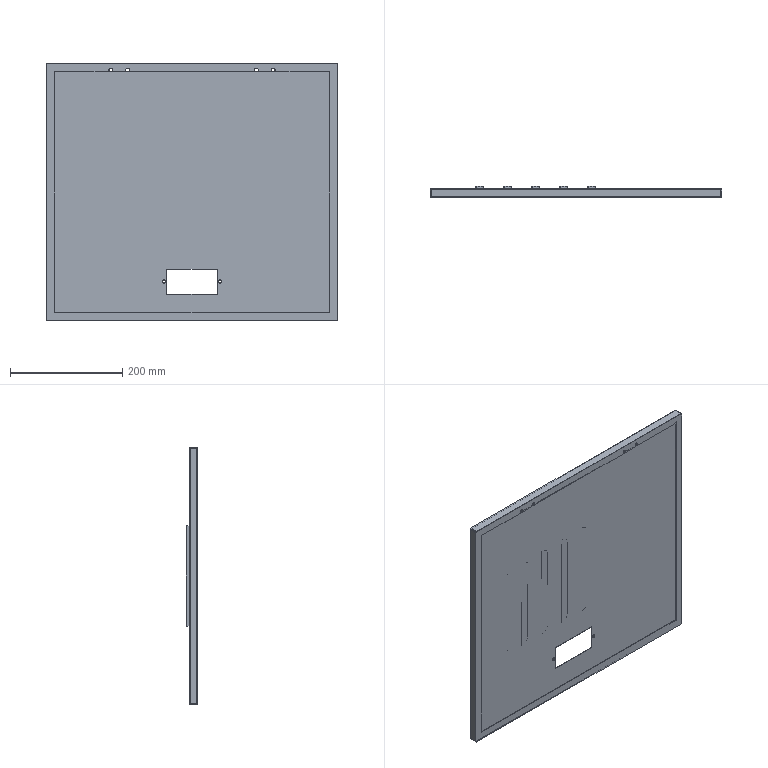Part | STEP file | 1 solid | 95 faces | box 520 x 20 x 460 mm | volume 497373 mm3 | plane 61 | cylinder 34 | commonest cylinder face diameters 6.5 x16 24 x10 4 x4 6 x4